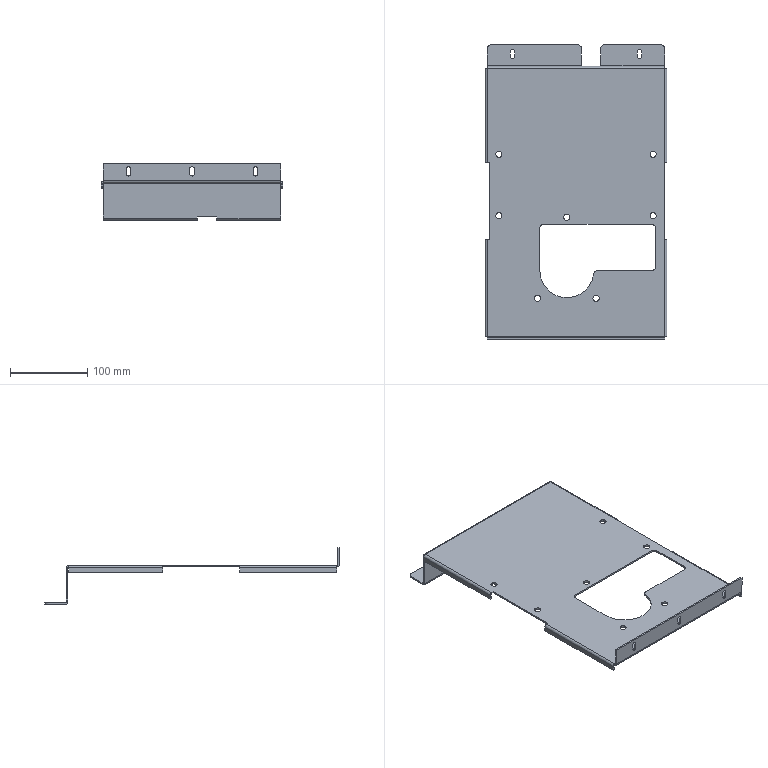Part | SolidWorks | features ICE 7, EdgeFlange 4, Fillet 2, SMBaseFlange 2, FlatPattern 1, MirrorPattern 1, SheetMetal 1 | 1 solid | 127 faces | box 236 x 382 x 73.5 mm | volume 191072 mm3 | plane 75 | cylinder 52 | commonest cylinder face diameters 6 x21 8 x14 2 x8 10 x8 70 x1